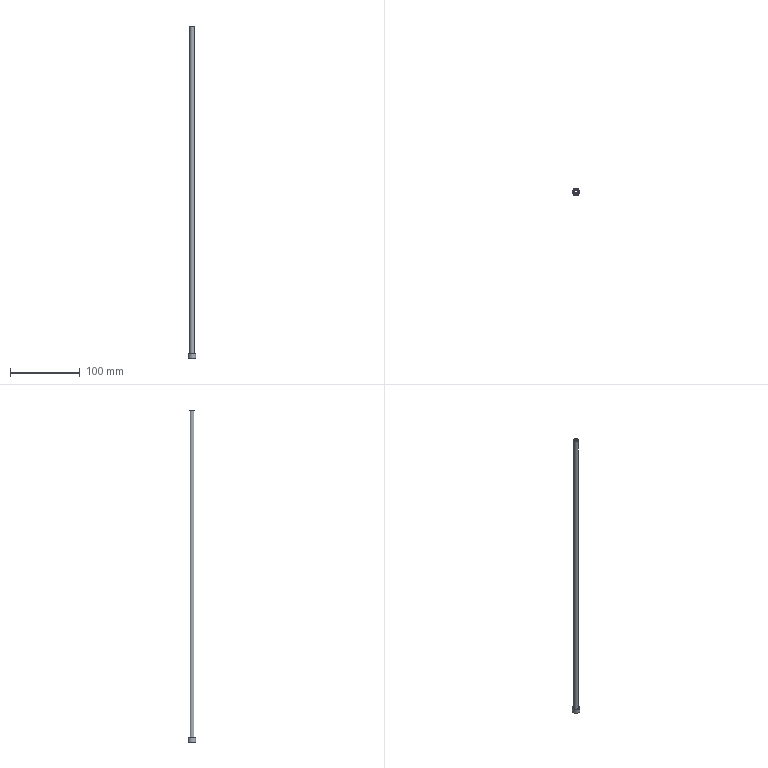Part | STEP file | solid 18 | 1 solid | 6 faces | box 11 x 11 x 477.132 mm | volume 11113 mm3 | cylinder 3 | plane 3 | commonest cylinder face diameters 4.5 x1 7 x1 11 x1